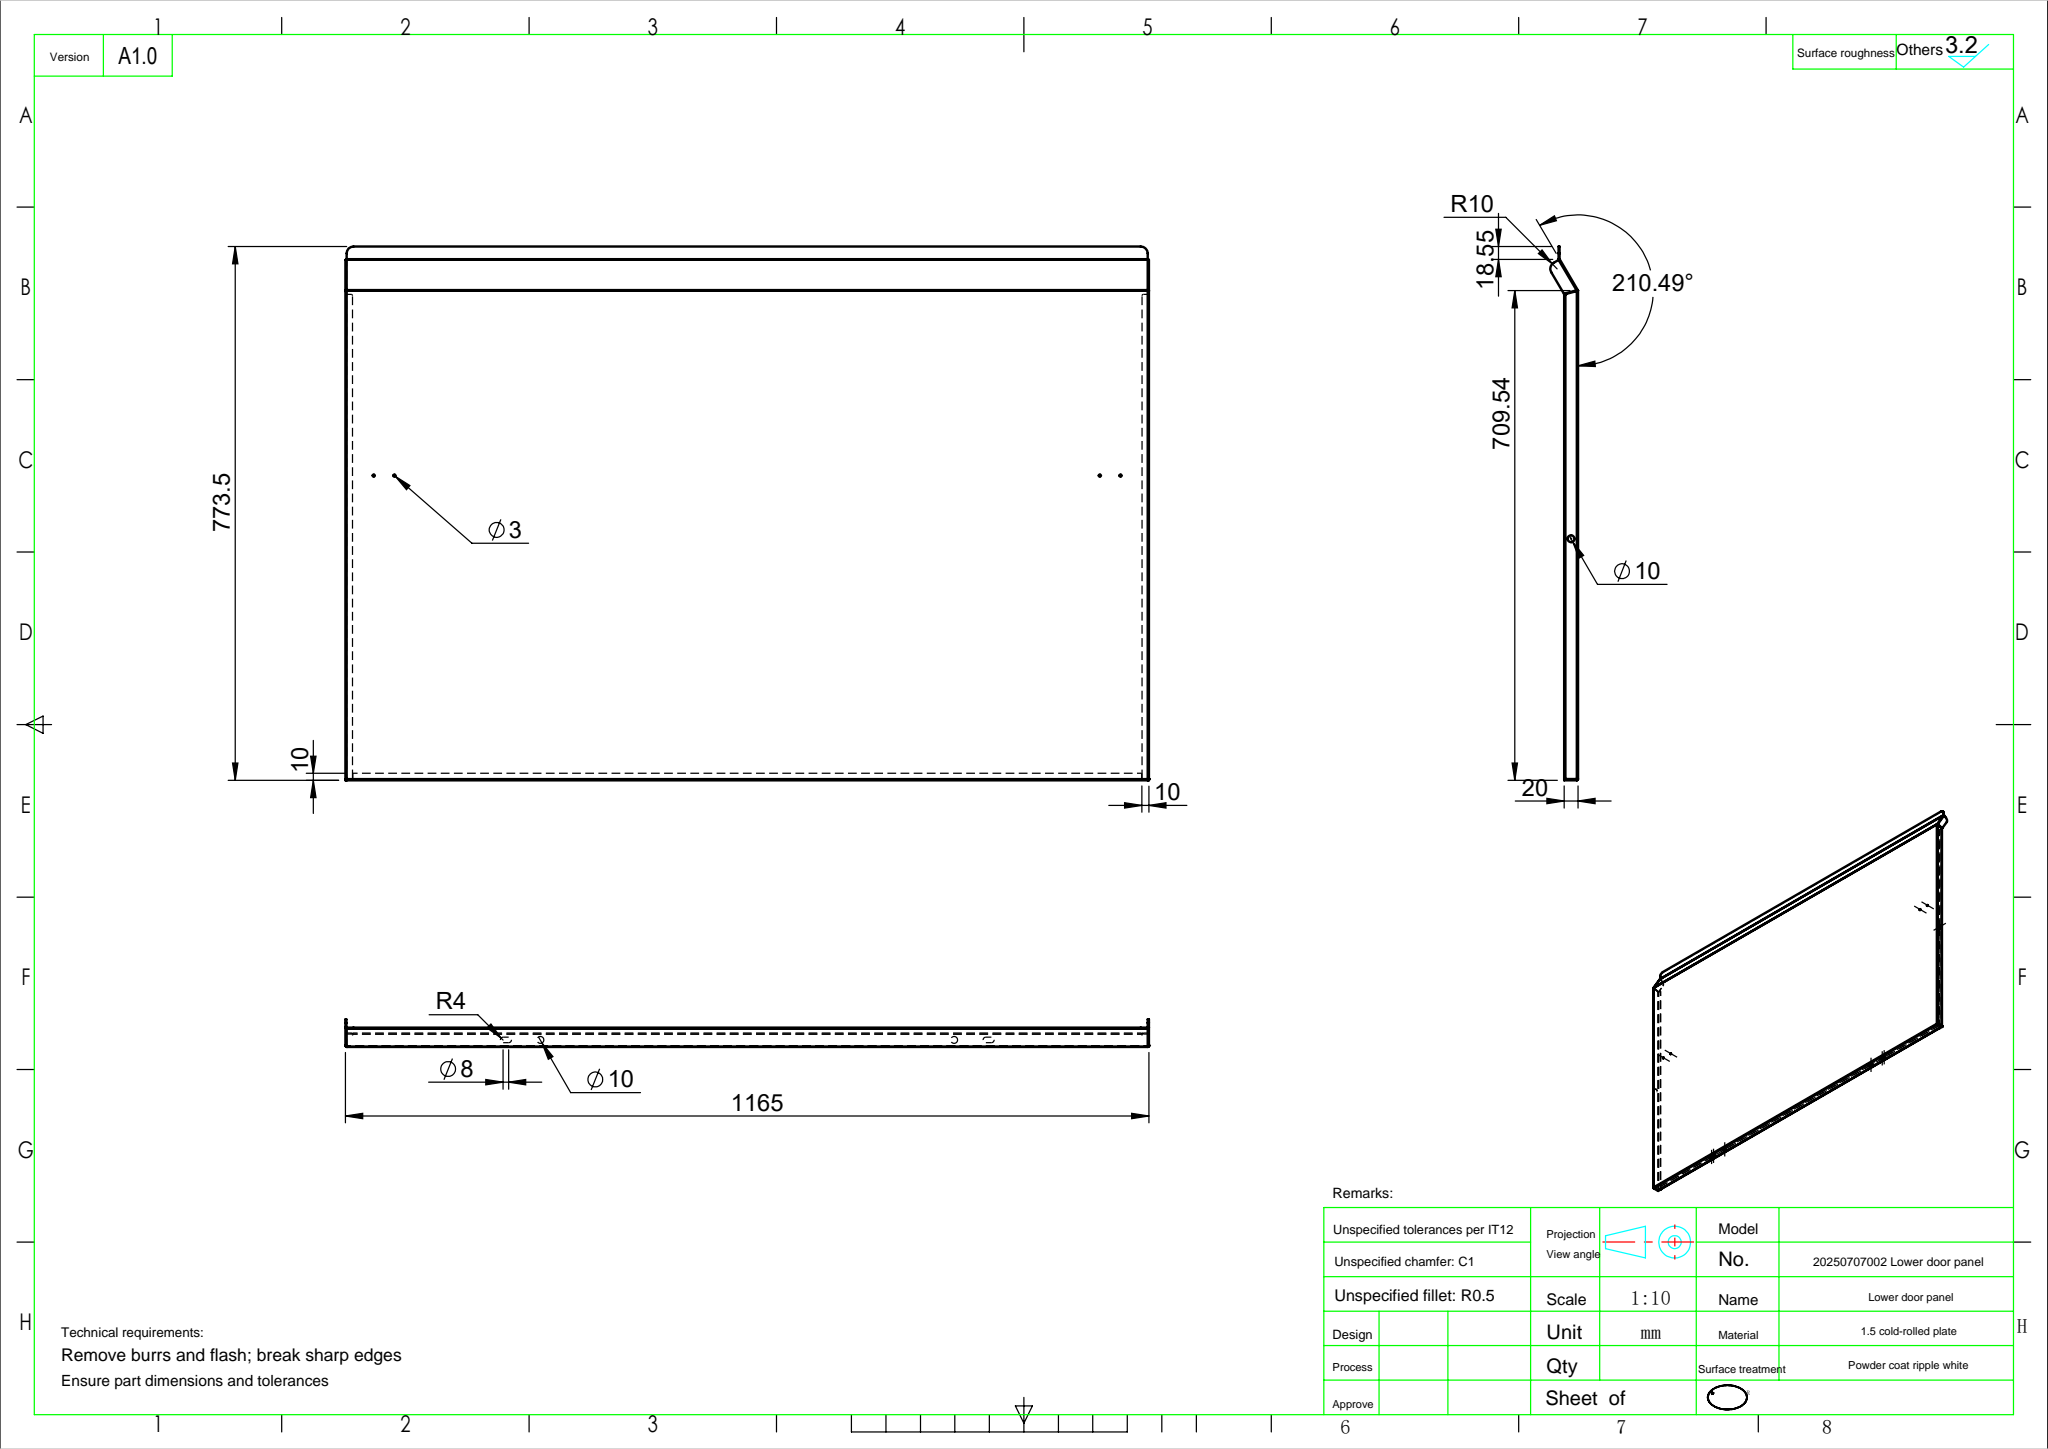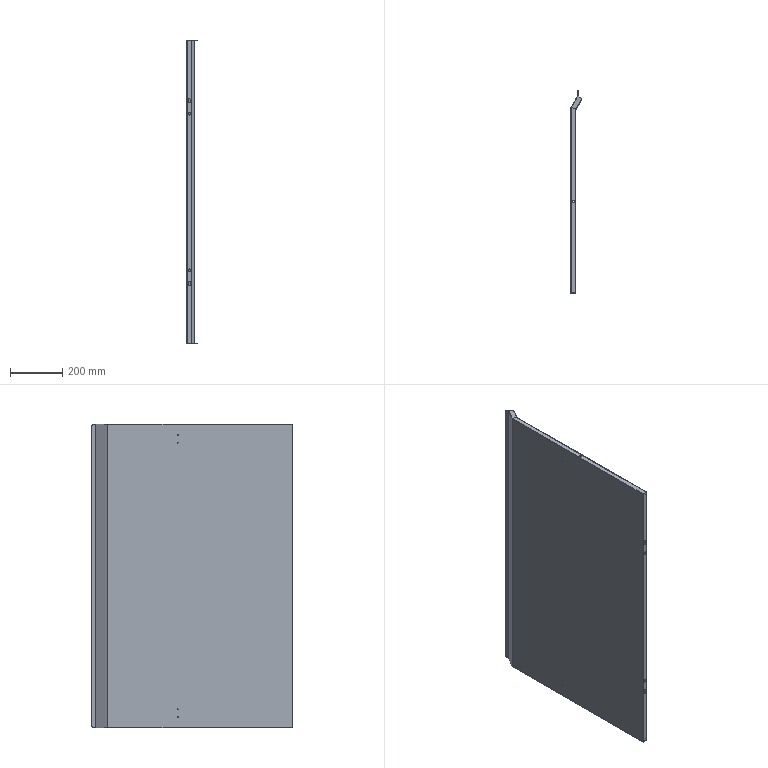Part | SolidWorks | features EdgeFlange 3, Fillet 2, ICE 2, CornerFeat 1, FlatPattern 1, HoleWzd 1, SMBaseFlange 1, SheetMetal 1 | 1 solid | 137 faces | box 40.015 x 773.5 x 1165 mm | volume 1466617 mm3 | plane 80 | cylinder 53 | spline 4 | commonest cylinder face diameters 0.4 x10 3.4 x10 3 x8 10 x8 8 x6 20 x5